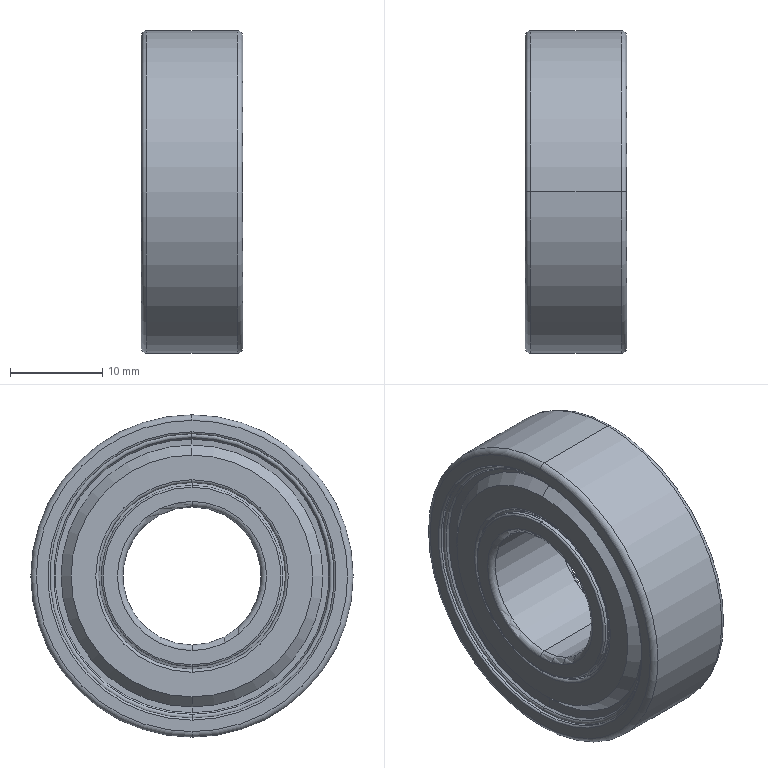Part | STEP file | HI_BAY6202ZZ^BFU71-6202ZZ-L40-S15_Idler roller assembly (direct encoder) | 1 solid | 132 faces | box 11 x 35 x 35 mm | volume 6855 mm3 | torus 48 | cone 40 | cylinder 32 | plane 12 | commonest cylinder face diameters 18.8 x4 19.7 x4 20.3 x4 20.9 x4 21.1 x4 28.9 x4